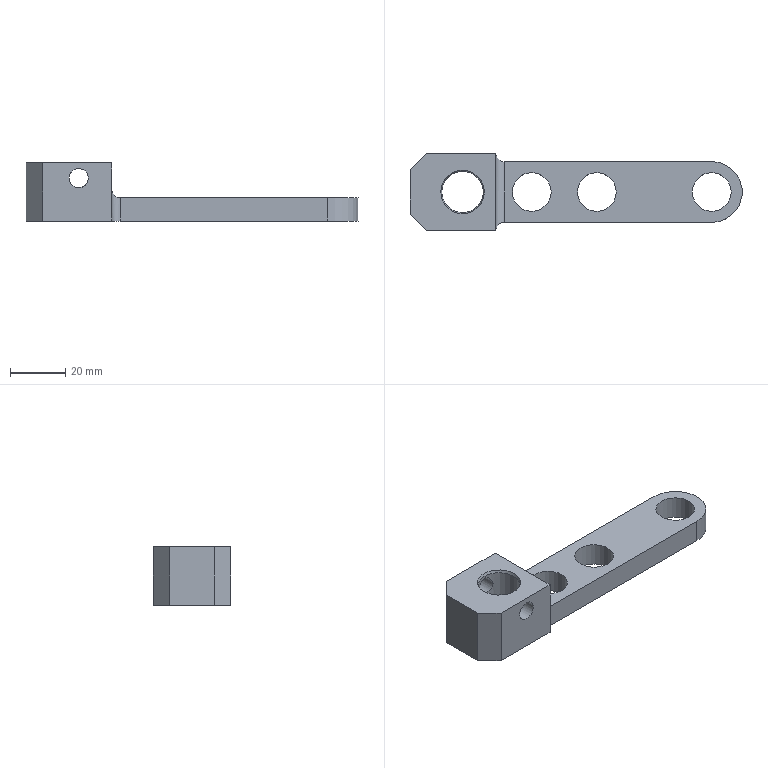NC program | NX | posted with a generic post | part box 120 x 28 x 21 mm
Lines 3458 to 4754 of 4754:
(低壁铣光面_1 , TOOL : D6-18-D6-50-3T-精)
N6914 T06 M6
N6916 G54
N6918 G17 G0 G90 X3.986 Y-12.5 B0. C0. S4500 M3
N6920 G43 Z6. H6
N6922 Z3.
N6924 G94 G1 Z0. F700.
N6926 X-0.257
N6928 X-34.
N6930 Y-8.483
N6932 X3.
N6934 Y-4.467
N6936 X-34.
N6938 Y-0.45
N6940 X3.
N6942 Y3.567
N6944 X-34.
N6946 Y7.583
N6948 X3.
N6950 Y9.243
N6952 X0.643 Y11.6
N6954 X-34.
N6956 X-37.
N6958 Z3.
N6960 G0 Z6.
N6962 X-118.5 Y-14.098
N6964 Z-9.5
N6966 G1 Z-12.5
N6968 Y-10.283
N6970 Y10.283
N6972 G2 X-114.211 Y12.994 R14.
N6974 G1 Y-12.994
N6976 G3 X-109.921 Y-13.97 R14.
N6978 G1 Y13.97
N6980 G2 X-109. Y14. R14.
N6982 G1 X-105.632
N6984 Y-14.
N6986 X-101.342
N6988 Y14.
N6990 X-97.053
N6992 Y-14.
N6994 X-92.763
N6996 Y14.
N6998 X-88.474
N7000 Y-14.
N7002 X-84.184
N7004 Y14.
N7006 X-79.895
N7008 Y-14.
N7010 X-75.605
N7012 Y14.
N7014 X-71.316
N7016 Y-14.
N7018 X-67.026
N7020 Y14.
N7022 X-62.737
N7024 Y-14.
N7026 X-58.447
N7028 Y14.
N7030 X-54.158
N7032 Y-14.
N7034 X-49.868
N7036 Y14.
N7038 X-45.579
N7040 Y-14.
N7042 X-41.289
N7044 Y14.
N7046 X-37.
N7048 Y-14.
N7050 Y-17.
N7052 Z-9.5
N7054 G0 Z6.
N7056 M5
(ZLEVEL_PROFILE_STEEP_1 , TOOL : 5R0.5)
N7058 T07 M6
N7060 G54
N7062 G17 G0 G90 X-38.632 Y-16.4 B0. C0. S4500 M3
N7064 G43 Z6. H7
N7066 Z0.55
N7068 G94 G1 Z-0.45 F2000.
N7070 X-37.4
N7072 G3 X-35. Y-14. R2.4
N7074 G1 Y14.
N7076 Z-0.5
N7078 Y-14.
N7080 Z-0.55
N7082 Y14.
N7084 Z-0.6
N7086 Y-14.
N7088 Z-0.65
N7090 Y14.
N7092 Z-0.7
N7094 Y-14.
N7096 Z-0.75
N7098 Y14.
N7100 Z-0.8
N7102 Y-14.
N7104 Z-0.85
N7106 Y14.
N7108 Z-0.9
N7110 Y-14.
N7112 Z-0.95
N7114 Y14.
N7116 Z-1.
N7118 Y-14.
N7120 Z-1.05
N7122 Y14.
N7124 Z-1.1
N7126 Y-14.
N7128 Z-1.15
N7130 Y14.
N7132 Z-1.2
N7134 Y-14.
N7136 Z-1.25
N7138 Y14.
N7140 Z-1.3
N7142 Y-14.
N7144 Z-1.35
N7146 Y14.
N7148 Z-1.4
N7150 Y-14.
N7152 Z-1.45
N7154 Y14.
N7156 Z-1.5
N7158 Y-14.
N7160 Z-1.55
N7162 Y14.
N7164 Z-1.6
N7166 Y-14.
N7168 Z-1.65
N7170 Y14.
N7172 Z-1.7
N7174 Y-14.
N7176 Z-1.75
N7178 Y14.
N7180 Z-1.8
N7182 Y-14.
N7184 Z-1.85
N7186 Y14.
N7188 Z-1.9
N7190 Y-14.
N7192 Z-1.95
N7194 Y14.
N7196 Z-2.
N7198 Y-14.
N7200 Z-2.05
N7202 Y14.
N7204 Z-2.1
N7206 Y-14.
N7208 Z-2.15
N7210 Y14.
N7212 Z-2.2
N7214 Y-14.
N7216 Z-2.25
N7218 Y14.
N7220 Z-2.3
N7222 Y-14.
N7224 Z-2.35
N7226 Y14.
N7228 Z-2.4
N7230 Y-14.
N7232 Z-2.45
N7234 Y14.
N7236 Z-2.5
N7238 Y-14.
N7240 Z-2.55
N7242 Y14.
N7244 Z-2.6
N7246 Y-14.
N7248 Z-2.65
N7250 Y14.
N7252 Z-2.7
N7254 Y-14.
N7256 Z-2.75
N7258 Y14.
N7260 Z-2.8
N7262 Y-14.
N7264 Z-2.85
N7266 Y14.
N7268 Z-2.9
N7270 Y-14.
N7272 Z-2.95
N7274 Y14.
N7276 Z-3.
N7278 Y-14.
N7280 Z-3.05
N7282 Y14.
N7284 Z-3.1
N7286 Y-14.
N7288 Z-3.15
N7290 Y14.
N7292 Z-3.2
N7294 Y-14.
N7296 Z-3.25
N7298 Y14.
N7300 Z-3.3
N7302 Y-14.
N7304 Z-3.35
N7306 Y14.
N7308 Z-3.4
N7310 Y-14.
N7312 Z-3.45
N7314 Y14.
N7316 Z-3.5
N7318 Y-14.
N7320 Z-3.55
N7322 Y14.
N7324 Z-3.6
N7326 Y-14.
N7328 Z-3.65
N7330 Y14.
N7332 Z-3.7
N7334 Y-14.
N7336 Z-3.75
N7338 Y14.
N7340 Z-3.8
N7342 Y-14.
N7344 Z-3.85
N7346 Y14.
N7348 Z-3.9
N7350 Y-14.
N7352 Z-3.95
N7354 Y14.
N7356 Z-4.
N7358 Y-14.
N7360 Z-4.05
N7362 Y14.
N7364 Z-4.1
N7366 Y-14.
N7368 Z-4.15
N7370 Y14.
N7372 Z-4.2
N7374 Y-14.
N7376 Z-4.25
N7378 Y14.
N7380 Z-4.3
N7382 Y-14.
N7384 Z-4.35
N7386 Y14.
N7388 Z-4.4
N7390 Y-14.
N7392 Z-4.45
N7394 Y14.
N7396 Z-4.5
N7398 Y-14.
N7400 Z-4.55
N7402 Y14.
N7404 Z-4.6
N7406 Y-14.
N7408 Z-4.65
N7410 Y14.
N7412 Z-4.7
N7414 Y-14.
N7416 Z-4.75
N7418 Y14.
N7420 Z-4.8
N7422 Y-14.
N7424 Z-4.85
N7426 Y14.
N7428 Z-4.9
N7430 Y-14.
N7432 Z-4.95
N7434 Y14.
N7436 Z-5.
N7438 Y-14.
N7440 Z-5.05
N7442 Y14.
N7444 Z-5.1
N7446 Y-14.
N7448 Z-5.15
N7450 Y14.
N7452 Z-5.2
N7454 Y-14.
N7456 Z-5.25
N7458 Y14.
N7460 Z-5.3
N7462 Y-14.
N7464 Z-5.35
N7466 Y14.
N7468 Z-5.4
N7470 Y-14.
N7472 Z-5.45
N7474 Y14.
N7476 Z-5.5
N7478 Y-14.
N7480 Z-5.55
N7482 Y14.
N7484 Z-5.6
N7486 Y-14.
N7488 Z-5.65
N7490 Y14.
N7492 Z-5.7
N7494 Y-14.
N7496 Z-5.75
N7498 Y14.
N7500 Z-5.8
N7502 Y-14.
N7504 Z-5.85
N7506 Y14.
N7508 Z-5.9
N7510 Y-14.
N7512 Z-5.95
N7514 Y14.
N7516 Z-6.
N7518 Y-14.
N7520 Z-6.05
N7522 Y14.
N7524 Z-6.1
N7526 Y-14.
N7528 Z-6.15
N7530 Y14.
N7532 Z-6.2
N7534 Y-14.
N7536 Z-6.25
N7538 Y14.
N7540 Z-6.3
N7542 Y-14.
N7544 Z-6.35
N7546 Y14.
N7548 Z-6.4
N7550 Y-14.
N7552 Z-6.45
N7554 Y14.
N7556 Z-6.5
N7558 Y-14.
N7560 Z-6.55
N7562 Y14.
N7564 Z-6.6
N7566 Y-14.
N7568 Z-6.65
N7570 Y14.
N7572 Z-6.7
N7574 Y-14.
N7576 Z-6.75
N7578 Y14.
N7580 Z-6.8
N7582 Y-14.
N7584 Z-6.85
N7586 Y14.
N7588 Z-6.9
N7590 Y-14.
N7592 Z-6.95
N7594 Y14.
N7596 Z-7.
N7598 Y-14.
N7600 Z-7.05
N7602 Y14.
N7604 Z-7.1
N7606 Y-14.
N7608 Z-7.15
N7610 Y14.
N7612 Z-7.2
N7614 Y-14.
N7616 Z-7.25
N7618 Y14.
N7620 Z-7.3
N7622 Y-14.
N7624 Z-7.35
N7626 Y14.
N7628 Z-7.4
N7630 Y-14.
N7632 Z-7.45
N7634 Y14.
N7636 Z-7.5
N7638 Y-14.
N7640 Z-7.55
N7642 Y14.
N7644 Z-7.6
N7646 Y-14.
N7648 Z-7.65
N7650 Y14.
N7652 Z-7.7
N7654 Y-14.
N7656 Z-7.75
N7658 Y14.
N7660 Z-7.8
N7662 Y-14.
N7664 Z-7.85
N7666 Y14.
N7668 Z-7.9
N7670 Y-14.
N7672 Z-7.95
N7674 Y14.
N7676 Z-8.
N7678 Y-14.
N7680 Z-8.05
N7682 Y14.
N7684 Z-8.1
N7686 Y-14.
N7688 Z-8.15
N7690 Y14.
N7692 Z-8.2
N7694 Y-14.
N7696 Z-8.25
N7698 Y14.
N7700 Z-8.3
N7702 Y-14.
N7704 Z-8.35
N7706 Y14.
N7708 Z-8.4
N7710 Y-14.
N7712 Z-8.45
N7714 Y14.
N7716 Z-8.5
N7718 Y-14.
N7720 Z-8.55
N7722 Y14.
N7724 Z-8.6
N7726 Y-14.
N7728 Z-8.65
N7730 Y14.
N7732 Z-8.7
N7734 Y-14.
N7736 Z-8.75
N7738 Y14.
N7740 Z-8.8
N7742 Y-14.
N7744 Z-8.85
N7746 Y14.
N7748 Z-8.9
N7750 Y-14.
N7752 Z-8.95
N7754 Y14.
N7756 Z-9.
N7758 Y-14.
N7760 Z-9.05
N7762 Y14.
N7764 Z-9.1
N7766 Y-14.
N7768 Z-9.15
N7770 Y14.
N7772 Z-9.2
N7774 Y-14.
N7776 Z-9.25
N7778 Y14.
N7780 Z-9.3
N7782 Y-14.
N7784 Z-9.35
N7786 Y14.
N7788 Z-9.4
N7790 Y-14.
N7792 Z-9.45
N7794 Y14.
N7796 Z-9.5
N7798 Y-14.
N7800 Z-9.55
N7802 Y14.
N7804 Z-9.6
N7806 Y-14.
N7808 Z-9.65
N7810 Y14.
N7812 Z-9.7
N7814 Y-14.
N7816 Z-9.75
N7818 Y14.
N7820 Z-9.8
N7822 Y-14.
N7824 Z-9.85
N7826 Y14.
N7828 Z-9.9
N7830 Y-13.847
N7832 X-35.002 Z-10.
N7834 Y13.818
N7836 X-35.004 Y13.77 Z-10.05
N7838 Y-13.712
N7840 X-35.008 Y-13.77 Z-10.1
N7842 Y13.77
N7844 X-35.012 Y13.712 Z-10.15
N7846 Y-13.655
N7848 X-35.017 Z-10.2
N7850 Y13.597
N7852 X-35.024 Z-10.25
N7854 Y-13.54
N7856 X-35.031 Y-13.501 Z-10.3
N7858 Y13.54
N7860 X-35.039 Y13.482 Z-10.35
N7862 Y-13.482
N7864 X-35.049 Y-13.425 Z-10.4
N7866 Y13.425
N7868 X-35.059 Y13.367 Z-10.45
N7870 Y-13.367
N7872 X-35.07 Y-13.309 Z-10.5
N7874 Y13.309
N7876 X-35.083 Y13.252 Z-10.55
N7878 Y-13.252
N7880 X-35.096 Y-13.194 Z-10.6
N7882 Y13.194
N7884 X-35.111 Y13.136 Z-10.65
N7886 Y-13.136
N7888 X-35.126 Y-13.079 Z-10.7
N7890 Y13.079
N7892 X-35.143 Y12.963 Z-10.75
N7894 Y-13.021
N7896 X-35.161 Y-12.904 Z-10.8
N7898 Y12.963
N7900 X-35.18 Y12.846 Z-10.85
N7902 Y-12.846
N7904 X-35.2 Z-10.9
N7906 Y12.846
N7908 X-35.221 Y12.79 Z-10.95
N7910 Y-12.733
N7912 X-35.244 Y-12.675 Z-11.
N7914 Y12.733
N7916 X-35.268 Y12.617 Z-11.05
N7918 Y-12.617
N7920 X-35.293 Y-12.558 Z-11.1
N7922 Y12.618
N7924 X-35.32 Y12.5 Z-11.15
N7926 Y-12.5
N7928 X-35.348 Y-12.501 Z-11.2
N7930 Y12.462
N7932 X-35.378 Y12.444 Z-11.25
N7934 Y-12.444
N7936 X-35.409 Y-12.388 Z-11.3
N7938 Y12.388
N7940 X-35.442 Y12.272 Z-11.35
N7942 Y-12.272
N7944 X-35.476 Z-11.4
N7946 Y12.213
N7948 X-35.513 Y12.155 Z-11.45
N7950 Y-12.213
N7952 X-35.531 Y-11.991 Z-11.475
N7954 X-35.551 Y-11.77 Z-11.5
N7956 Y12.155
N7958 X-35.591 Y12.099 Z-11.55
N7960 Y-12.099
N7962 X-35.633 Y-12.043 Z-11.6
N7964 Y12.043
N7966 X-35.677 Y11.985 Z-11.65
N7968 Y-11.985
N7970 X-35.724 Y-11.925 Z-11.7
N7972 Y11.925
N7974 X-35.773 Y11.866 Z-11.75
N7976 Y-11.866
N7978 X-35.825 Y-11.811 Z-11.8
N7980 Y11.811
N7982 X-35.88 Y11.755 Z-11.85
N7984 Y-11.755
N7986 X-35.939 Y-11.696 Z-11.9
N7988 Y11.696
N7990 X-36.001 Y11.636 Z-11.95
N7992 Y-11.637
N7994 X-36.067 Y-11.58 Z-12.
N7996 Y11.58
N7998 X-36.138 Y11.525 Z-12.05
N8000 Y-11.527
N8002 X-36.214 Y-11.469 Z-12.1
N8004 Y11.466
N8006 X-36.297 Y11.407 Z-12.15
N8008 Y-11.407
N8010 X-36.388 Y-11.351 Z-12.2
N8012 Y11.351
N8014 X-36.488 Y11.294 Z-12.25
N8016 Y-11.294
N8018 X-36.6 Y-11.235 Z-12.3
N8020 Y11.235
N8022 X-36.73 Y11.178 Z-12.35
N8024 Y-11.178
N8026 X-36.886 Y-11.12 Z-12.4
N8028 Y11.12
N8030 X-37.093 Y11.06 Z-12.45
N8032 Y-11.06
N8034 X-37.245 Y-11.036 Z-12.475
N8036 X-37.403 Y-11.01 Z-12.5
N8038 Y11.01
N8040 G3 X-39.803 Y13.41 R2.4
N8042 G1 X-41.029
N8044 Z-11.5
N8046 G0 Z6.
(ZLEVEL_PROFILE_STEEP_COPY , TOOL : 5R0.5)
N8048 X-17.594 Y1.39
N8050 Z1.201
N8052 G1 Z0.201 F1000.
N8054 X-17. Y1.977
N8056 G3 X-19. Y3.977 R2.
N8058 X-22.977 Y0. R3.977
N8060 X-19. Y3.977 R-3.977
N8062 G1 X-19.282 Y3.947 Z0.187
N8064 X-19.566 Y3.925 Z0.172
N8066 G3 X-19. Y3.966 R-3.966
N8068 G1 X-19.283 Y3.936 Z0.157
N8070 X-19.566 Y3.914 Z0.142
N8072 G3 X-19. Y3.955 R-3.955
N8074 G1 X-19.283 Y3.929 Z0.127
N8076 X-19.566 Y3.905 Z0.112
N8078 G3 X-19. Y3.946 R-3.946
N8080 G1 X-19.283 Y3.922 Z0.097
N8082 X-19.566 Y3.895 Z0.082
N8084 G3 X-19. Y3.936 R-3.936
N8086 G1 X-19.283 Y3.915 Z0.067
N8088 X-19.566 Y3.885 Z0.052
N8090 G3 X-19. Y3.926 R-3.925
N8092 G1 X-19.283 Y3.908 Z0.037
N8094 X-19.566 Y3.875 Z0.022
N8096 G3 X-19. Y3.916 R-3.916
N8098 G1 X-19.284 Y3.902 Z0.007
N8100 X-19.567 Y3.87 Z-0.007
N8102 G3 X-19. Y3.912 R-3.912
N8104 G1 X-19.283 Y3.895 Z-0.022
N8106 X-19.565 Y3.856 Z-0.037
N8108 G3 X-19. Y3.897 R-3.896
N8110 G1 X-19.284 Y3.888 Z-0.052
N8112 X-19.566 Y3.849 Z-0.067
N8114 G3 X-19. Y3.891 R-3.892
N8116 G1 X-19.284 Y3.882 Z-0.082
N8118 X-19.566 Y3.839 Z-0.097
N8120 G3 X-19. Y3.881 R-3.88
N8122 G1 X-19.285 Y3.875 Z-0.112
N8124 X-19.567 Y3.836 Z-0.127
N8126 G3 X-19. Y3.877 R-3.877
N8128 G1 X-19.284 Y3.869 Z-0.142
N8130 X-19.566 Y3.828 Z-0.157
N8132 G3 X-19. Y3.869 R-3.87
N8134 G1 X-19.284 Y3.852 Z-0.172
N8136 X-19.567 Y3.827 Z-0.187
N8138 G3 X-19. Y3.868 R-3.868
N8140 G1 X-19.283 Y3.847 Z-0.201
N8142 X-19.567 Y3.823 Z-0.216
N8144 G3 X-19. Y3.864 R-3.864
N8146 G1 X-19.283 Y3.843 Z-0.231
N8148 X-19.567 Y3.819 Z-0.246
N8150 G3 X-19. Y3.86 R-3.86
N8152 G1 X-19.283 Y3.839 Z-0.261
N8154 X-19.567 Y3.815 Z-0.276
N8156 G3 X-19. Y3.856 R-3.856
N8158 G1 X-19.283 Y3.835 Z-0.291
N8160 X-19.567 Y3.811 Z-0.306
N8162 G3 X-19. Y3.853 R-3.853
N8164 G1 X-19.283 Y3.831 Z-0.321
N8166 X-19.567 Y3.807 Z-0.336
N8168 G3 X-19.637 Y-3.816 R3.861
N8170 X-15.649 Y1.931 R3.886
N8172 X-19. Y3.851 R3.861
N8174 G1 X-19.283 Y3.827 Z-0.351
N8176 X-19.567 Y3.809 Z-0.366
N8178 G3 X-22.741 Y0.914 R3.851
N8180 G1 X-22.85 Y0.058
N8182 G3 X-15.259 Y-0.914 R3.851
N8184 G1 X-15.15 Y-0.058
N8186 G3 X-19. Y3.851 R3.851
N8188 G1 X-19.284 Y3.835 Z-0.381
N8190 X-19.566 Y3.798 Z-0.396
N8192 G3 X-20.455 Y3.553 R3.84
N8194 G1 X-20.789 Y3.398
N8196 G3 X-21.014 Y3.269 R3.84
N8198 G1 X-21.438 Y2.967
N8200 G3 X-22.386 Y1.811 R3.84
N8202 G1 X-22.555 Y1.452
N8204 G3 X-22.803 Y0.529 R3.84
N8206 G1 X-22.836 Y0.169
N8208 G3 X-22.553 Y-1.455 R3.84
N8210 G1 X-22.389 Y-1.805
N8212 G3 X-22.254 Y-2.039 R3.84
N8214 G1 X-21.967 Y-2.438
N8216 G3 X-20.811 Y-3.386 R3.84
N8218 G1 X-20.452 Y-3.555
N8220 G3 X-19.529 Y-3.803 R3.84
N8222 G1 X-19.118 Y-3.838
N8224 G3 X-17.545 Y-3.553 R3.84
N8226 G1 X-17.195 Y-3.39
N8228 G3 X-16.986 Y-3.27 R3.84
N8230 G1 X-16.562 Y-2.967
N8232 G3 X-15.614 Y-1.811 R3.84
N8234 G1 X-15.445 Y-1.452
N8236 G3 X-15.197 Y-0.529 R3.84
N8238 G1 X-15.164 Y-0.169
N8240 G3 X-15.447 Y1.455 R3.84
N8242 G1 X-15.602 Y1.789
N8244 G3 X-15.731 Y2.014 R3.84
N8246 G1 X-16.033 Y2.438
N8248 G3 X-17.189 Y3.386 R3.84
N8250 G1 X-17.548 Y3.555
N8252 G3 X-19. Y3.84 R3.84
N8254 G1 X-19.284 Y3.824 Z-0.41
N8256 X-19.566 Y3.787 Z-0.425
N8258 G3 X-19. Y3.829 R-3.829
N8260 G1 X-19.284 Y3.813 Z-0.44
N8262 X-19.566 Y3.776 Z-0.455
N8264 G3 X-19. Y3.818 R-3.818
N8266 G1 X-19.283 Y3.802 Z-0.47
N8268 X-19.566 Y3.765 Z-0.485
N8270 G3 X-19. Y3.807 R-3.807
N8272 G1 X-19.283 Y3.791 Z-0.5
N8274 X-19.566 Y3.754 Z-0.515
N8276 G3 X-19. Y3.796 R-3.796
N8278 G1 X-19.283 Y3.78 Z-0.53
N8280 X-19.566 Y3.743 Z-0.545
N8282 G3 X-19. Y3.786 R-3.786
N8284 G1 X-19.283 Y3.77 Z-0.56
N8286 X-19.566 Y3.732 Z-0.575
N8288 G3 X-19. Y3.775 R-3.775
N8290 G1 X-19.283 Y3.759 Z-0.59
N8292 X-19.566 Y3.721 Z-0.604
N8294 G3 X-19. Y3.764 R-3.764
N8296 G1 X-19.283 Y3.748 Z-0.619
N8298 X-19.566 Y3.71 Z-0.634
N8300 G3 X-19. Y3.753 R-3.753
N8302 G1 X-19.283 Y3.737 Z-0.649
N8304 X-19.566 Y3.699 Z-0.664
N8306 G3 X-19. Y3.742 R-3.742
N8308 G1 X-19.283 Y3.726 Z-0.679
N8310 X-19.566 Y3.688 Z-0.694
N8312 G3 X-19. Y3.731 R-3.731
N8314 G1 X-19.283 Y3.715 Z-0.709
N8316 X-19.566 Y3.677 Z-0.724
N8318 G3 X-19. Y3.72 R-3.72
N8320 G1 X-19.283 Y3.704 Z-0.739
N8322 X-19.565 Y3.666 Z-0.754
N8324 G3 X-19. Y3.71 R-3.71
N8326 G1 X-19.283 Y3.693 Z-0.769
N8328 X-19.565 Y3.655 Z-0.784
N8330 G3 X-19. Y3.699 R-3.699
N8332 G1 X-19.283 Y3.682 Z-0.799
N8334 X-19.565 Y3.644 Z-0.813
N8336 G3 X-19. Y3.688 R-3.688
N8338 G1 X-19.283 Y3.671 Z-0.828
N8340 X-19.565 Y3.633 Z-0.843
N8342 G3 X-19. Y3.677 R-3.677
N8344 G1 X-19.283 Y3.661 Z-0.858
N8346 X-19.565 Y3.622 Z-0.873
N8348 G3 X-19. Y3.666 R-3.666
N8350 G1 X-19.283 Y3.65 Z-0.888
N8352 X-19.565 Y3.611 Z-0.903
N8354 G3 X-19. Y3.655 R-3.655
N8356 G1 X-19.283 Y3.639 Z-0.918
N8358 X-19.565 Y3.6 Z-0.933
N8360 G3 X-19. Y3.644 R-3.644
N8362 G1 X-19.283 Y3.628 Z-0.948
N8364 X-19.565 Y3.589 Z-0.963
N8366 G3 X-19. Y3.633 R-3.633
N8368 G1 X-19.283 Y3.617 Z-0.978
N8370 X-19.565 Y3.578 Z-0.993
N8372 G3 X-19. Y3.623 R-3.623
N8374 G1 X-19.283 Y3.606 Z-1.007
N8376 X-19.565 Y3.567 Z-1.022
N8378 G3 X-19. Y3.612 R-3.612
N8380 G1 X-19.283 Y3.595 Z-1.037
N8382 X-19.565 Y3.556 Z-1.052
N8384 G3 X-19. Y3.601 R-3.601
N8386 G1 X-19.283 Y3.584 Z-1.067
N8388 X-19.565 Y3.545 Z-1.082
N8390 G3 X-19. Y3.59 R-3.59
N8392 G1 X-19.283 Y3.573 Z-1.097
N8394 X-19.565 Y3.534 Z-1.112
N8396 G3 X-19. Y3.579 R-3.579
N8398 G1 X-19.283 Y3.562 Z-1.127
N8400 X-19.565 Y3.523 Z-1.142
N8402 G3 X-19. Y3.568 R-3.568
N8404 G1 X-19.283 Y3.543 Z-1.157
N8406 X-19.565 Y3.512 Z-1.172
N8408 G3 X-20.146 Y3.368 R3.557
N8410 G1 X-20.654 Y3.139
N8412 X-20.693 Y3.129
N8414 G3 X-21.561 Y2.469 R3.557
N8416 G1 X-21.646 Y2.378
N8418 G3 X-22.256 Y1.434 R3.557
N8420 G1 X-22.258 Y1.401
N8422 X-22.376 Y1.122
N8424 G3 X-22.548 Y0.263 R3.557
N8426 G1 X-22.557 Y0.081
N8428 G3 X-22.368 Y-1.146 R3.557
N8430 G1 X-22.139 Y-1.673
N8432 X-22.05 Y-1.831
N8434 X-21.978 Y-1.947
N8436 G3 X-21.863 Y-2.112 R3.557
N8438 G1 X-21.792 Y-2.204
N8440 G3 X-21.66 Y-2.362 R3.557
N8442 G1 X-21.469 Y-2.561
N8444 X-21.378 Y-2.646
N8446 G3 X-20.477 Y-3.236 R3.557
N8448 G1 X-20.429 Y-3.246
N8450 X-20.122 Y-3.376
N8452 G3 X-19.263 Y-3.548 R3.557
N8454 G1 X-19.081 Y-3.557
N8456 G3 X-17.854 Y-3.368 R3.557
N8458 G1 X-17.327 Y-3.139
N8460 G3 X-16.888 Y-2.863 R3.557
N8462 G1 X-16.796 Y-2.792
N8464 G3 X-16.439 Y-2.469 R3.557
N8466 G1 X-16.354 Y-2.378
N8468 G3 X-15.764 Y-1.477 R3.557
N8470 G1 X-15.754 Y-1.429
N8472 X-15.624 Y-1.121
N8474 G3 X-15.452 Y-0.263 R3.557
N8476 G1 X-15.443 Y-0.081
N8478 G3 X-15.632 Y1.146 R3.557
N8480 G1 X-15.861 Y1.654
N8482 X-15.871 Y1.693
N8484 G3 X-16.531 Y2.561 R3.557
N8486 G1 X-16.622 Y2.646
N8488 G3 X-17.566 Y3.256 R3.557
N8490 G1 X-17.598 Y3.258
N8492 X-17.879 Y3.376
N8494 G3 X-18.737 Y3.548 R3.557
N8496 G1 X-19. Y3.557
N8498 X-19.282 Y3.523 Z-1.187
N8500 X-19.565 Y3.501 Z-1.201
N8502 G3 X-19. Y3.547 R-3.547
N8504 G1 X-19.281 Y3.51 Z-1.216
N8506 X-19.562 Y3.469 Z-1.231
N8508 G3 X-19. Y3.514 R-3.514
N8510 G1 X-19.283 Y3.491 Z-1.246
N8512 X-19.564 Y3.45 Z-1.261
N8514 G3 X-19. Y3.496 R-3.496
N8516 G1 X-19.283 Y3.472 Z-1.276
N8518 X-19.564 Y3.432 Z-1.291
N8520 G3 X-19. Y3.478 R-3.478
N8522 G1 X-19.282 Y3.454 Z-1.306
N8524 X-19.564 Y3.414 Z-1.321
N8526 G3 X-19. Y3.46 R-3.46
N8528 G1 X-19.282 Y3.435 Z-1.336
N8530 X-19.563 Y3.393 Z-1.351
N8532 G3 X-19. Y3.439 R-3.441
N8534 G1 X-19.283 Y3.416 Z-1.366
N8536 X-19.564 Y3.378 Z-1.381
N8538 G3 X-19. Y3.425 R-3.425
N8540 G1 X-19.282 Y3.398 Z-1.396
N8542 X-19.564 Y3.362 Z-1.41
N8544 G3 X-22.398 Y-0.297 R3.411
N8546 X-16.284 Y-2.064 R3.412
N8548 X-19. Y3.408 R3.411
N8550 G1 X-19.282 Y3.38 Z-1.425
N8552 X-19.564 Y3.345 Z-1.44
N8554 G3 X-20.616 Y2.983 R3.396
N8556 G1 X-20.755 Y2.904
N8558 X-20.814 Y2.886
N8560 G3 X-22.091 Y1.376 R3.551
N8562 X-18.312 Y-3.317 R3.376
N8564 X-16.301 Y-2.064 R3.376
N8566 X-19. Y3.392 R3.396
N8568 G1 X-19.283 Y3.367 Z-1.455
N8570 X-19.565 Y3.332 Z-1.47
N8572 G3 X-22.302 Y0.688 R3.363
N8574 X-18.312 Y-3.302 R3.358
N8576 X-15.698 Y0.688 R3.35
N8578 X-17.608 Y3.074 R3.325
N8580 X-19. Y3.378 R3.363
N8582 G1 X-19.283 Y3.353 Z-1.485
N8584 X-19.565 Y3.319 Z-1.5
N8586 G3 X-21.24 Y-2.508 R3.365
N8588 X-15.804 Y-1.056 R3.357
N8590 X-19.565 Y3.319 R3.365
N8592 X-21.2 Y1.011 R2.
N8594 G1 X-20.239 Y0.571
N8596 Z-0.5
N8598 G0 Z6.
N8600 M5
(PLANAR_MILL_3 , TOOL : 倒角D4-90度)
N8602 T05 M6
N8604 G54
N8606 G17 G0 G90 X-34.5 Y-2. B0. C0. S3500 M3
N8608 G43 Z6. H5
N8610 Z0.5
N8612 G94 G1 Z-1.5 F800.
N8614 G3 X-32.5 Y0. R2.
N8616 G1 Y14.
N8618 G2 X-31. Y15.5 R1.5
N8620 G1 X-6.
N8622 G2 X-4.939 Y15.061 R1.5
N8624 G1 X1.061 Y9.061
N8626 G2 X1.5 Y8. R1.5
N8628 G1 Y-8.
N8630 G2 X1.061 Y-9.061 R1.5
N8632 G1 X-4.939 Y-15.061
N8634 G2 X-6. Y-15.5 R1.5
N8636 G1 X-31.
N8638 G2 X-32.5 Y-14. R1.5
N8640 G1 Y0.
N8642 G3 X-34.5 Y2. R2.
N8644 G1 Z0.5
N8646 G0 Z6.
(PLANAR_MILL_3_COPY_1 , TOOL : 倒角D4-90度)
N8648 X-35. Y-14.5
N8650 Z-12.
N8652 G1 Z-14.
N8654 G3 X-37. Y-12.5 R2.
N8656 G1 X-109.
N8658 G2 X-121.5 Y0. R12.5
N8660 X-109. Y12.5 R12.5
N8662 G1 X-37.
N8664 G3 X-35. Y14.5 R2.
N8666 G1 Z-12.
N8668 G0 Z6.
(PLANAR_MILL_3_COPY , TOOL : 倒角D4-90度)
N8670 X-46.872 Y2.
N8672 Z-12.
N8674 G1 Z-14.
N8676 X-47.5
N8678 G3 X-49.5 Y0. R2.
N8680 X-44. Y-5.5 R5.5
N8682 X-49.5 Y0. R-5.5
N8684 X-47.5 Y-2. R2.
N8686 G1 X-46.872
N8688 Z-12.
N8690 G0 Z6.
N8692 X-70.372 Y2.
N8694 Z-12.
N8696 G1 Z-14.
N8698 X-71.
N8700 G3 X-73. Y0. R2.
N8702 X-67.5 Y-5.5 R5.5
N8704 X-73. Y0. R-5.5
N8706 X-71. Y-2. R2.
N8708 G1 X-70.372
N8710 Z-12.
N8712 G0 Z6.
N8714 X-111.872 Y2.
N8716 Z-12.
N8718 G1 Z-14.
N8720 X-112.5
N8722 G3 X-114.5 Y0. R2.
N8724 X-109. Y-5.5 R5.5
N8726 X-114.5 Y0. R-5.5
N8728 X-112.5 Y-2. R2.
N8730 G1 X-111.872
N8732 Z-12.
N8734 G0 Z6.
N8736 M5
(HOLE_MILLING , TOOL : D8-25-D8-60-3T-精)
N8738 T08 M6
N8740 G54
N8742 G17 G0 G90 X-44. Y0. B0. C0. S3000 M3
N8744 G43 Z6. H8
N8746 Z-9.5
N8748 G94 G3 X-45.475 Y1.475 R1.475 F800.
N8750 X-46.95 Y0. R1.475
N8752 X-46.95 Y0. Z-9.8 I2.95 J0.
N8754 X-46.95 Y0. Z-10.1 I2.95 J0.
N8756 X-46.95 Y0. Z-10.4 I2.95 J0.
N8758 X-46.95 Y0. Z-10.7 I2.95 J0.
N8760 X-46.95 Y0. Z-11. I2.95 J0.
N8762 X-46.95 Y0. Z-11.3 I2.95 J0.
N8764 X-46.95 Y0. Z-11.6 I2.95 J0.
N8766 X-46.95 Y0. Z-11.9 I2.95 J0.
N8768 X-46.95 Y0. Z-12.2 I2.95 J0.
N8770 X-46.95 Y0. Z-12.5 I2.95 J0.
N8772 X-46.95 Y0. Z-12.8 I2.95 J0.
N8774 X-46.95 Y0. Z-13.1 I2.95 J0.
N8776 X-46.95 Y0. Z-13.4 I2.95 J0.
N8778 X-46.95 Y0. Z-13.7 I2.95 J0.
N8780 X-46.95 Y0. Z-14. I2.95 J0.
N8782 X-46.95 Y0. Z-14.3 I2.95 J0.
N8784 X-46.95 Y0. Z-14.6 I2.95 J0.
N8786 X-46.95 Y0. Z-14.9 I2.95 J0.
N8788 X-46.95 Y0. Z-15.2 I2.95 J0.
N8790 X-46.95 Y0. Z-15.5 I2.95 J0.
N8792 X-46.95 Y0. Z-15.8 I2.95 J0.
N8794 X-46.95 Y0. Z-16.1 I2.95 J0.
N8796 X-46.95 Y0. Z-16.4 I2.95 J0.
N8798 X-46.95 Y0. Z-16.7 I2.95 J0.
N8800 X-46.95 Y0. Z-17. I2.95 J0.
N8802 X-46.95 Y0. Z-17.3 I2.95 J0.
N8804 X-46.95 Y0. Z-17.6 I2.95 J0.
N8806 X-46.95 Y0. Z-17.9 I2.95 J0.
N8808 X-46.95 Y0. Z-18.2 I2.95 J0.
N8810 X-46.95 Y0. Z-18.5 I2.95 J0.
N8812 X-46.95 Y0. Z-18.8 I2.95 J0.
N8814 X-46.95 Y0. Z-19.1 I2.95 J0.
N8816 X-46.95 Y0. Z-19.4 I2.95 J0.
N8818 X-46.95 Y0. Z-19.7 I2.95 J0.
N8820 X-46.95 Y0. Z-20. I2.95 J0.
N8822 X-46.95 Y0. Z-20.3 I2.95 J0.
N8824 X-46.95 Y0. Z-20.6 I2.95 J0.
N8826 X-46.95 Y0. Z-20.9 I2.95 J0.
N8828 X-46.95 Y0. Z-21.2 I2.95 J0.
N8830 X-46.95 Y0. Z-21.5 I2.95 J0.
N8832 X-44. Y-2.95 R2.95
N8834 X-46.95 Y0. R-2.95
N8836 X-45.475 Y-1.475 R1.475
N8838 X-44. Y0. R1.475
N8840 G0 Z6.
N8842 X-67.5
N8844 Z-9.5
N8846 G3 X-68.975 Y1.475 R1.475
N8848 X-70.45 Y0. R1.475
N8850 X-70.45 Y0. Z-9.8 I2.95 J0.
N8852 X-70.45 Y0. Z-10.1 I2.95 J0.
N8854 X-70.45 Y0. Z-10.4 I2.95 J0.
N8856 X-70.45 Y0. Z-10.7 I2.95 J0.
N8858 X-70.45 Y0. Z-11. I2.95 J0.
N8860 X-70.45 Y0. Z-11.3 I2.95 J0.
N8862 X-70.45 Y0. Z-11.6 I2.95 J0.
N8864 X-70.45 Y0. Z-11.9 I2.95 J0.
N8866 X-70.45 Y0. Z-12.2 I2.95 J0.
N8868 X-70.45 Y0. Z-12.5 I2.95 J0.
N8870 X-70.45 Y0. Z-12.8 I2.95 J0.
N8872 X-70.45 Y0. Z-13.1 I2.95 J0.
N8874 X-70.45 Y0. Z-13.4 I2.95 J0.
N8876 X-70.45 Y0. Z-13.7 I2.95 J0.
N8878 X-70.45 Y0. Z-14. I2.95 J0.
N8880 X-70.45 Y0. Z-14.3 I2.95 J0.
N8882 X-70.45 Y0. Z-14.6 I2.95 J0.
N8884 X-70.45 Y0. Z-14.9 I2.95 J0.
N8886 X-70.45 Y0. Z-15.2 I2.95 J0.
N8888 X-70.45 Y0. Z-15.5 I2.95 J0.
N8890 X-70.45 Y0. Z-15.8 I2.95 J0.
N8892 X-70.45 Y0. Z-16.1 I2.95 J0.
N8894 X-70.45 Y0. Z-16.4 I2.95 J0.
N8896 X-70.45 Y0. Z-16.7 I2.95 J0.
N8898 X-70.45 Y0. Z-17. I2.95 J0.
N8900 X-70.45 Y0. Z-17.3 I2.95 J0.
N8902 X-70.45 Y0. Z-17.6 I2.95 J0.
N8904 X-70.45 Y0. Z-17.9 I2.95 J0.
N8906 X-70.45 Y0. Z-18.2 I2.95 J0.
N8908 X-70.45 Y0. Z-18.5 I2.95 J0.
N8910 X-70.45 Y0. Z-18.8 I2.95 J0.
N8912 X-70.45 Y0. Z-19.1 I2.95 J0.
N8914 X-70.45 Y0. Z-19.4 I2.95 J0.
N8916 X-70.45 Y0. Z-19.7 I2.95 J0.
N8918 X-70.45 Y0. Z-20. I2.95 J0.
N8920 X-70.45 Y0. Z-20.3 I2.95 J0.
N8922 X-70.45 Y0. Z-20.6 I2.95 J0.
N8924 X-70.45 Y0. Z-20.9 I2.95 J0.
N8926 X-70.45 Y0. Z-21.2 I2.95 J0.
N8928 X-70.45 Y0. Z-21.5 I2.95 J0.
N8930 X-67.5 Y-2.95 R2.95
N8932 X-70.45 Y0. R-2.95
N8934 X-68.975 Y-1.475 R1.475
N8936 X-67.5 Y0. R1.475
N8938 G0 Z6.
N8940 X-109.
N8942 Z-9.5
N8944 G3 X-110.475 Y1.475 R1.475
N8946 X-111.95 Y0. R1.475
N8948 X-111.95 Y0. Z-9.8 I2.95 J0.
N8950 X-111.95 Y0. Z-10.1 I2.95 J0.
N8952 X-111.95 Y0. Z-10.4 I2.95 J0.
N8954 X-111.95 Y0. Z-10.7 I2.95 J0.
N8956 X-111.95 Y0. Z-11. I2.95 J0.
N8958 X-111.95 Y0. Z-11.3 I2.95 J0.
N8960 X-111.95 Y0. Z-11.6 I2.95 J0.
N8962 X-111.95 Y0. Z-11.9 I2.95 J0.
N8964 X-111.95 Y0. Z-12.2 I2.95 J0.
N8966 X-111.95 Y0. Z-12.5 I2.95 J0.
N8968 X-111.95 Y0. Z-12.8 I2.95 J0.
N8970 X-111.95 Y0. Z-13.1 I2.95 J0.
N8972 X-111.95 Y0. Z-13.4 I2.95 J0.
N8974 X-111.95 Y0. Z-13.7 I2.95 J0.
N8976 X-111.95 Y0. Z-14. I2.95 J0.
N8978 X-111.95 Y0. Z-14.3 I2.95 J0.
N8980 X-111.95 Y0. Z-14.6 I2.95 J0.
N8982 X-111.95 Y0. Z-14.9 I2.95 J0.
N8984 X-111.95 Y0. Z-15.2 I2.95 J0.
N8986 X-111.95 Y0. Z-15.5 I2.95 J0.
N8988 X-111.95 Y0. Z-15.8 I2.95 J0.
N8990 X-111.95 Y0. Z-16.1 I2.95 J0.
N8992 X-111.95 Y0. Z-16.4 I2.95 J0.
N8994 X-111.95 Y0. Z-16.7 I2.95 J0.
N8996 X-111.95 Y0. Z-17. I2.95 J0.
N8998 X-111.95 Y0. Z-17.3 I2.95 J0.
N9000 X-111.95 Y0. Z-17.6 I2.95 J0.
N9002 X-111.95 Y0. Z-17.9 I2.95 J0.
N9004 X-111.95 Y0. Z-18.2 I2.95 J0.
N9006 X-111.95 Y0. Z-18.5 I2.95 J0.
N9008 X-111.95 Y0. Z-18.8 I2.95 J0.
N9010 X-111.95 Y0. Z-19.1 I2.95 J0.
N9012 X-111.95 Y0. Z-19.4 I2.95 J0.
N9014 X-111.95 Y0. Z-19.7 I2.95 J0.
N9016 X-111.95 Y0. Z-20. I2.95 J0.
N9018 X-111.95 Y0. Z-20.3 I2.95 J0.
N9020 X-111.95 Y0. Z-20.6 I2.95 J0.
N9022 X-111.95 Y0. Z-20.9 I2.95 J0.
N9024 X-111.95 Y0. Z-21.2 I2.95 J0.
N9026 X-111.95 Y0. Z-21.5 I2.95 J0.
N9028 X-109. Y-2.95 R2.95
N9030 X-111.95 Y0. R-2.95
N9032 X-110.475 Y-1.475 R1.475
N9034 X-109. Y0. R1.475
N9036 G0 Z6.
(HOLE_MILLING_1 , TOOL : D8-25-D8-60-3T-精)
N9038 X-19.
N9040 Z3.
N9042 G3 X-20.725 Y1.725 R1.725
N9044 X-22.45 Y0. R1.725
N9046 X-22.45 Y0. Z2.7 I3.45 J0.
N9048 X-22.45 Y0. Z2.4 I3.45 J0.
N9050 X-22.45 Y0. Z2.1 I3.45 J0.
N9052 X-22.45 Y0. Z1.8 I3.45 J0.
N9054 X-22.45 Y0. Z1.5 I3.45 J0.
N9056 X-22.45 Y0. Z1.2 I3.45 J0.
N9058 X-22.45 Y0. Z0.9 I3.45 J0.
N9060 X-22.45 Y0. Z0.6 I3.45 J0.
N9062 X-22.45 Y0. Z0.3 I3.45 J0.
N9064 X-22.45 Y0. Z0. I3.45 J0.
N9066 X-22.45 Y0. Z-0.3 I3.45 J0.
N9068 X-22.45 Y0. Z-0.6 I3.45 J0.
N9070 X-22.45 Y0. Z-0.9 I3.45 J0.
N9072 X-22.45 Y0. Z-1.2 I3.45 J0.
N9074 X-22.45 Y0. Z-1.5 I3.45 J0.
N9076 X-22.45 Y0. Z-1.8 I3.45 J0.
N9078 X-22.45 Y0. Z-2.1 I3.45 J0.
N9080 X-22.45 Y0. Z-2.4 I3.45 J0.
N9082 X-22.45 Y0. Z-2.7 I3.45 J0.
N9084 X-22.45 Y0. Z-3. I3.45 J0.
N9086 X-22.45 Y0. Z-3.3 I3.45 J0.
N9088 X-22.45 Y0. Z-3.6 I3.45 J0.
N9090 X-22.45 Y0. Z-3.9 I3.45 J0.
N9092 X-22.45 Y0. Z-4.2 I3.45 J0.
N9094 X-22.45 Y0. Z-4.5 I3.45 J0.
N9096 X-22.45 Y0. Z-4.8 I3.45 J0.
N9098 X-22.45 Y0. Z-5.1 I3.45 J0.
N9100 X-22.45 Y0. Z-5.4 I3.45 J0.
N9102 X-22.45 Y0. Z-5.7 I3.45 J0.
N9104 X-22.45 Y0. Z-6. I3.45 J0.
N9106 X-22.45 Y0. Z-6.3 I3.45 J0.
N9108 X-22.45 Y0. Z-6.6 I3.45 J0.
N9110 X-22.45 Y0. Z-6.9 I3.45 J0.
N9112 X-22.45 Y0. Z-7.2 I3.45 J0.
N9114 X-22.45 Y0. Z-7.5 I3.45 J0.
N9116 X-22.45 Y0. Z-7.8 I3.45 J0.
N9118 X-22.45 Y0. Z-8.1 I3.45 J0.
N9120 X-22.45 Y0. Z-8.4 I3.45 J0.
N9122 X-22.45 Y0. Z-8.7 I3.45 J0.
N9124 X-22.45 Y0. Z-9. I3.45 J0.
N9126 X-22.45 Y0. Z-9.3 I3.45 J0.
N9128 X-22.45 Y0. Z-9.6 I3.45 J0.
N9130 X-22.45 Y0. Z-9.9 I3.45 J0.
N9132 X-22.45 Y0. Z-10.2 I3.45 J0.
N9134 X-22.45 Y0. Z-10.5 I3.45 J0.
N9136 X-22.45 Y0. Z-10.8 I3.45 J0.
N9138 X-22.45 Y0. Z-11.1 I3.45 J0.
N9140 X-22.45 Y0. Z-11.4 I3.45 J0.
N9142 X-22.45 Y0. Z-11.7 I3.45 J0.
N9144 X-22.45 Y0. Z-12. I3.45 J0.
N9146 X-22.45 Y0. Z-12.3 I3.45 J0.
N9148 X-22.45 Y0. Z-12.6 I3.45 J0.
N9150 X-22.45 Y0. Z-12.9 I3.45 J0.
N9152 X-22.45 Y0. Z-13.2 I3.45 J0.
N9154 X-22.45 Y0. Z-13.5 I3.45 J0.
N9156 X-22.45 Y0. Z-13.8 I3.45 J0.
N9158 X-22.45 Y0. Z-14.1 I3.45 J0.
N9160 X-22.45 Y0. Z-14.4 I3.45 J0.
N9162 X-22.45 Y0. Z-14.7 I3.45 J0.
N9164 X-22.45 Y0. Z-15. I3.45 J0.
N9166 X-22.45 Y0. Z-15.3 I3.45 J0.
N9168 X-22.45 Y0. Z-15.6 I3.45 J0.
N9170 X-22.45 Y0. Z-15.9 I3.45 J0.
N9172 X-22.45 Y0. Z-16.2 I3.45 J0.
N9174 X-22.45 Y0. Z-16.5 I3.45 J0.
N9176 X-22.45 Y0. Z-16.8 I3.45 J0.
N9178 X-22.45 Y0. Z-17.1 I3.45 J0.
N9180 X-22.45 Y0. Z-17.4 I3.45 J0.
N9182 X-22.45 Y0. Z-17.7 I3.45 J0.
N9184 X-22.45 Y0. Z-18. I3.45 J0.
N9186 X-22.45 Y0. Z-18.3 I3.45 J0.
N9188 X-22.45 Y0. Z-18.6 I3.45 J0.
N9190 X-22.45 Y0. Z-18.9 I3.45 J0.
N9192 X-22.45 Y0. Z-19.2 I3.45 J0.
N9194 X-22.45 Y0. Z-19.5 I3.45 J0.
N9196 X-22.45 Y0. Z-19.8 I3.45 J0.
N9198 X-22.45 Y0. Z-20.1 I3.45 J0.
N9200 X-22.45 Y0. Z-20.4 I3.45 J0.
N9202 X-22.45 Y0. Z-20.7 I3.45 J0.
N9204 X-22.45 Y0. Z-21. I3.45 J0.
N9206 X-22.45 Y0. Z-21.3 I3.45 J0.
N9208 X-17.275 Y2.988 Z-21.5 R-3.45
N9210 X-21.988 Y1.725 R3.45
N9212 X-17.275 Y2.988 R-3.45
N9214 X-19.631 Y2.356 R1.725
N9216 X-19. Y0. R1.725
N9218 G0 Z6.
(PLANAR_MILL_4 , TOOL : D8-25-D8-60-3T-精)
N9220 X-18.087 Y-1.207
N9222 Z-19.5
N9224 G1 Z-21.5 F200.
N9226 G41 X-17.487 Y-2. D8
N9228 G3 X-15.487 Y0. R2.
N9230 X-19. Y3.513 R3.513
N9232 X-15.487 Y0. R-3.513
N9234 X-17.487 Y2. R2.
N9236 G40
N9238 G1 X-17.684 Y1.965
N9240 Y-1.965
N9242 G41 X-17.487 Y-2.
N9244 G3 X-15.487 Y0. R2.
N9246 X-19. Y3.513 R3.513
N9248 X-15.487 Y0. R-3.513
N9250 X-17.487 Y2. R2.
N9252 G40
N9254 G1 X-17.684 Y1.965
N9256 Y-1.965
N9258 G41 X-17.487 Y-2.
N9260 G3 X-15.487 Y0. R2.
N9262 X-19. Y3.513 R3.513
N9264 X-15.487 Y0. R-3.513
N9266 X-17.487 Y2. R2.
N9268 G40
N9270 G1 X-18.087 Y1.207
N9272 Z-19.5
N9274 G0 Z6.
(PLANAR_MILL_4_COPY , TOOL : D8-25-D8-60-3T-精)
N9276 X-44.447 Y0.894
N9278 Z-19.5
N9280 G1 Z-21.5
N9282 G41 X-45. Y2.
N9284 G3 X-47. Y0. R2.
N9286 X-44. Y-3. R3.
N9288 X-47. Y0. R-3.
N9290 X-45. Y-2. R2.
N9292 G40
N9294 G1 X-44.803 Y-1.965
N9296 Y1.965
N9298 G41 X-45. Y2.
N9300 G3 X-47. Y0. R2.
N9302 X-44. Y-3. R3.
N9304 X-47. Y0. R-3.
N9306 X-45. Y-2. R2.
N9308 G40
N9310 G1 X-44.803 Y-1.965
N9312 Y1.965
N9314 G41 X-45. Y2.
N9316 G3 X-47. Y0. R2.
N9318 X-44. Y-3. R3.
N9320 X-47. Y0. R-3.
N9322 X-45. Y-2. R2.
N9324 G40
N9326 G1 X-44.447 Y-0.894
N9328 Z-19.5
N9330 G0 Z6.
N9332 X-67.947 Y0.894
N9334 Z-19.5
N9336 G1 Z-21.5
N9338 G41 X-68.5 Y2.
N9340 G3 X-70.5 Y0. R2.
N9342 X-67.5 Y-3. R3.
N9344 X-70.5 Y0. R-3.
N9346 X-68.5 Y-2. R2.
N9348 G40
N9350 G1 X-68.303 Y-1.965
N9352 Y1.965
N9354 G41 X-68.5 Y2.
N9356 G3 X-70.5 Y0. R2.
N9358 X-67.5 Y-3. R3.
N9360 X-70.5 Y0. R-3.
N9362 X-68.5 Y-2. R2.
N9364 G40
N9366 G1 X-68.303 Y-1.965
N9368 Y1.965
N9370 G41 X-68.5 Y2.
N9372 G3 X-70.5 Y0. R2.
N9374 X-67.5 Y-3. R3.
N9376 X-70.5 Y0. R-3.
N9378 X-68.5 Y-2. R2.
N9380 G40
N9382 G1 X-67.947 Y-0.894
N9384 Z-19.5
N9386 G0 Z6.
N9388 X-109.447 Y0.894
N9390 Z-19.5
N9392 G1 Z-21.5
N9394 G41 X-110. Y2.
N9396 G3 X-112. Y0. R2.
N9398 X-109. Y-3. R3.
N9400 X-112. Y0. R-3.
N9402 X-110. Y-2. R2.
N9404 G40
N9406 G1 X-109.803 Y-1.965
N9408 Y1.965
N9410 G41 X-110. Y2.
N9412 G3 X-112. Y0. R2.
N9414 X-109. Y-3. R3.
N9416 X-112. Y0. R-3.
N9418 X-110. Y-2. R2.
N9420 G40
N9422 G1 X-109.803 Y-1.965
N9424 Y1.965
N9426 G41 X-110. Y2.
N9428 G3 X-112. Y0. R2.
N9430 X-109. Y-3. R3.
N9432 X-112. Y0. R-3.
N9434 X-110. Y-2. R2.
N9436 G40
N9438 G1 X-109.447 Y-0.894
N9440 Z-19.5
N9442 G0 Z6.
N9444 M5
N9446 M2